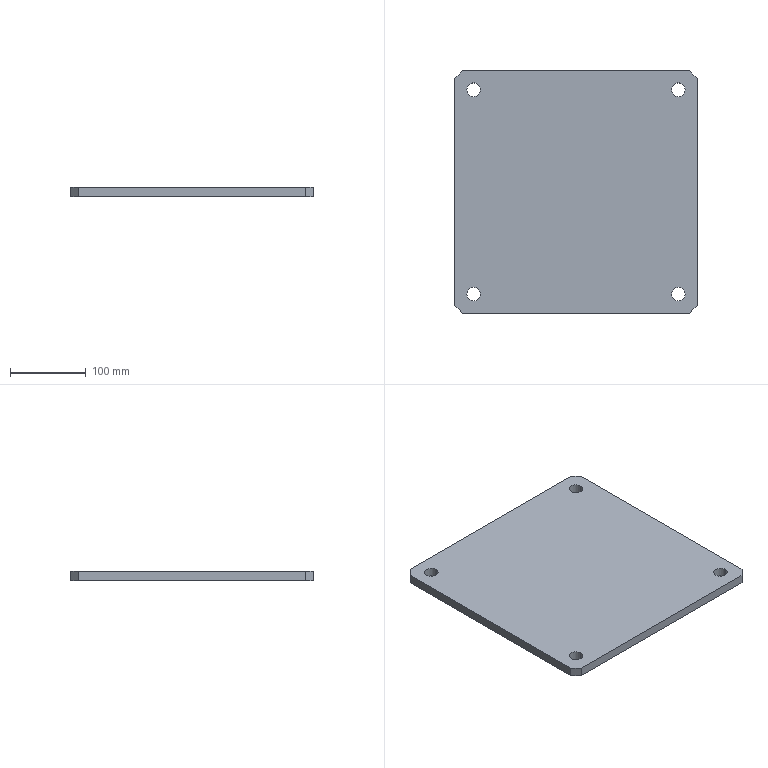Part | STEP file | PN_0109 Mount electronic clip vibrating disc base plate | 1 solid | 18 faces | box 320 x 320 x 12 mm | volume 1214185 mm3 | plane 10 | cylinder 8 | commonest cylinder face diameters 18 x8
STEP:
#1=CARTESIAN_POINT('',(0.,0.,0.));
#2=DIRECTION('',(0.,0.,1.));
#3=DIRECTION('',(1.,0.,0.));
#4=AXIS2_PLACEMENT_3D('',#1,#2,#3);
#5=CARTESIAN_POINT('',(144.,-135.,0.));
#6=VERTEX_POINT('',#5);
#7=CARTESIAN_POINT('',(144.,-135.,12.));
#8=VERTEX_POINT('',#7);
#9=CARTESIAN_POINT('',(144.,-135.,12.));
#10=DIRECTION('',(0.,0.,1.));
#11=VECTOR('',#10,1.);
#12=LINE('',#9,#11);
#13=CARTESIAN_POINT('',(135.,-135.,12.));
#14=DIRECTION('',(0.,0.,1.));
#15=DIRECTION('',(1.,0.,0.));
#16=AXIS2_PLACEMENT_3D('',#13,#14,#15);
#17=CYLINDRICAL_SURFACE('',#16,9.);
#18=CARTESIAN_POINT('',(6.283,0.));
#19=DIRECTION('',(0.,1.));
#20=VECTOR('',#19,1.);
#21=LINE('',#18,#20);
#22=(GEOMETRIC_REPRESENTATION_CONTEXT(2)PARAMETRIC_REPRESENTATION_CONTEXT()REPRESENTATION_CONTEXT('',''));
#23=DEFINITIONAL_REPRESENTATION('',(#21),#22);
#24=PCURVE('',#17,#23);
#25=CARTESIAN_POINT('',(135.,-135.,12.));
#26=DIRECTION('',(0.,0.,1.));
#27=DIRECTION('',(1.,0.,0.));
#28=AXIS2_PLACEMENT_3D('',#25,#26,#27);
#29=CYLINDRICAL_SURFACE('',#28,9.);
#30=CARTESIAN_POINT('',(0.,0.));
#31=DIRECTION('',(0.,1.));
#32=VECTOR('',#31,1.);
#33=LINE('',#30,#32);
#34=(GEOMETRIC_REPRESENTATION_CONTEXT(2)PARAMETRIC_REPRESENTATION_CONTEXT()REPRESENTATION_CONTEXT('',''));
#35=DEFINITIONAL_REPRESENTATION('',(#33),#34);
#36=PCURVE('',#29,#35);
#37=SURFACE_CURVE('',#12,(#24,#36),.PCURVE_S1.);
#38=EDGE_CURVE('',#6,#8,#37,.T.);
#39=ORIENTED_EDGE('',*,*,#38,.T.);
#40=CARTESIAN_POINT('',(126.,-135.,12.));
#41=VERTEX_POINT('',#40);
#42=CARTESIAN_POINT('',(135.,-135.,12.));
#43=DIRECTION('',(0.,0.,1.));
#44=DIRECTION('',(1.,0.,0.));
#45=AXIS2_PLACEMENT_3D('',#42,#43,#44);
#46=CIRCLE('',#45,9.);
#47=CARTESIAN_POINT('',(0.,0.));
#48=DIRECTION('',(1.,0.));
#49=VECTOR('',#48,1.);
#50=LINE('',#47,#49);
#51=(GEOMETRIC_REPRESENTATION_CONTEXT(2)PARAMETRIC_REPRESENTATION_CONTEXT()REPRESENTATION_CONTEXT('',''));
#52=DEFINITIONAL_REPRESENTATION('',(#50),#51);
#53=PCURVE('',#17,#52);
#54=CARTESIAN_POINT('',(0.,0.,12.));
#55=DIRECTION('',(0.,0.,-1.));
#56=DIRECTION('',(-1.,0.,0.));
#57=AXIS2_PLACEMENT_3D('',#54,#55,#56);
#58=PLANE('',#57);
#59=CARTESIAN_POINT('',(-144.,-135.));
#60=CARTESIAN_POINT('',(-144.,-119.412));
#61=CARTESIAN_POINT('',(-130.5,-127.206));
#62=CARTESIAN_POINT('',(-117.,-135.));
#63=CARTESIAN_POINT('',(-130.5,-142.794));
#64=CARTESIAN_POINT('',(-144.,-150.588));
#65=CARTESIAN_POINT('',(-144.,-135.));
#66=(BOUNDED_CURVE()B_SPLINE_CURVE(2,(#59,#60,#61,#62,#63,#64,#65),.UNSPECIFIED.,.T.,.F.)B_SPLINE_CURVE_WITH_KNOTS((1,2,2,2,2,1),(-2.094,0.,2.094,4.189,6.283,8.378),.UNSPECIFIED.)CURVE()GEOMETRIC_REPRESENTATION_ITEM()RATIONAL_B_SPLINE_CURVE((1.,0.5,1.,0.5,1.,0.5,1.))REPRESENTATION_ITEM(''));
#67=(GEOMETRIC_REPRESENTATION_CONTEXT(2)PARAMETRIC_REPRESENTATION_CONTEXT()REPRESENTATION_CONTEXT('',''));
#68=DEFINITIONAL_REPRESENTATION('',(#66),#67);
#69=PCURVE('',#58,#68);
#70=SURFACE_CURVE('',#46,(#53,#69),.PCURVE_S1.);
#71=EDGE_CURVE('',#41,#8,#70,.T.);
#72=ORIENTED_EDGE('',*,*,#71,.F.);
#73=CARTESIAN_POINT('',(126.,-135.,0.));
#74=VERTEX_POINT('',#73);
#75=CARTESIAN_POINT('',(126.,-135.,12.));
#76=DIRECTION('',(0.,0.,1.));
#77=VECTOR('',#76,1.);
#78=LINE('',#75,#77);
#79=CARTESIAN_POINT('',(3.142,0.));
#80=DIRECTION('',(0.,1.));
#81=VECTOR('',#80,1.);
#82=LINE('',#79,#81);
#83=(GEOMETRIC_REPRESENTATION_CONTEXT(2)PARAMETRIC_REPRESENTATION_CONTEXT()REPRESENTATION_CONTEXT('',''));
#84=DEFINITIONAL_REPRESENTATION('',(#82),#83);
#85=PCURVE('',#17,#84);
#86=CARTESIAN_POINT('',(3.142,0.));
#87=DIRECTION('',(0.,1.));
#88=VECTOR('',#87,1.);
#89=LINE('',#86,#88);
#90=(GEOMETRIC_REPRESENTATION_CONTEXT(2)PARAMETRIC_REPRESENTATION_CONTEXT()REPRESENTATION_CONTEXT('',''));
#91=DEFINITIONAL_REPRESENTATION('',(#89),#90);
#92=PCURVE('',#29,#91);
#93=SURFACE_CURVE('',#78,(#85,#92),.PCURVE_S1.);
#94=EDGE_CURVE('',#74,#41,#93,.T.);
#95=ORIENTED_EDGE('',*,*,#94,.F.);
#96=CARTESIAN_POINT('',(135.,-135.,0.));
#97=DIRECTION('',(0.,0.,-1.));
#98=DIRECTION('',(-1.,0.,0.));
#99=AXIS2_PLACEMENT_3D('',#96,#97,#98);
#100=CIRCLE('',#99,9.);
#101=CARTESIAN_POINT('',(9.425,-12.));
#102=DIRECTION('',(-1.,0.));
#103=VECTOR('',#102,1.);
#104=LINE('',#101,#103);
#105=(GEOMETRIC_REPRESENTATION_CONTEXT(2)PARAMETRIC_REPRESENTATION_CONTEXT()REPRESENTATION_CONTEXT('',''));
#106=DEFINITIONAL_REPRESENTATION('',(#104),#105);
#107=PCURVE('',#17,#106);
#108=CARTESIAN_POINT('',(0.,0.,0.));
#109=DIRECTION('',(0.,0.,-1.));
#110=DIRECTION('',(-1.,0.,0.));
#111=AXIS2_PLACEMENT_3D('',#108,#109,#110);
#112=PLANE('',#111);
#113=CARTESIAN_POINT('',(-135.,-135.));
#114=DIRECTION('',(1.,0.));
#115=AXIS2_PLACEMENT_2D('',#113,#114);
#116=CIRCLE('',#115,9.);
#117=(GEOMETRIC_REPRESENTATION_CONTEXT(2)PARAMETRIC_REPRESENTATION_CONTEXT()REPRESENTATION_CONTEXT('',''));
#118=DEFINITIONAL_REPRESENTATION('',(#116),#117);
#119=PCURVE('',#112,#118);
#120=SURFACE_CURVE('',#100,(#107,#119),.PCURVE_S1.);
#121=EDGE_CURVE('',#6,#74,#120,.T.);
#122=ORIENTED_EDGE('',*,*,#121,.F.);
#123=EDGE_LOOP('',(#39,#72,#95,#122));
#124=FACE_BOUND('',#123,.F.);
#125=ADVANCED_FACE('',(#124),#17,.F.);
#126=CARTESIAN_POINT('',(144.,135.,0.));
#127=VERTEX_POINT('',#126);
#128=CARTESIAN_POINT('',(144.,135.,12.));
#129=VERTEX_POINT('',#128);
#130=CARTESIAN_POINT('',(144.,135.,12.));
#131=DIRECTION('',(0.,0.,1.));
#132=VECTOR('',#131,1.);
#133=LINE('',#130,#132);
#134=CARTESIAN_POINT('',(135.,135.,12.));
#135=DIRECTION('',(0.,0.,1.));
#136=DIRECTION('',(1.,0.,0.));
#137=AXIS2_PLACEMENT_3D('',#134,#135,#136);
#138=CYLINDRICAL_SURFACE('',#137,9.);
#139=CARTESIAN_POINT('',(6.283,0.));
#140=DIRECTION('',(0.,1.));
#141=VECTOR('',#140,1.);
#142=LINE('',#139,#141);
#143=(GEOMETRIC_REPRESENTATION_CONTEXT(2)PARAMETRIC_REPRESENTATION_CONTEXT()REPRESENTATION_CONTEXT('',''));
#144=DEFINITIONAL_REPRESENTATION('',(#142),#143);
#145=PCURVE('',#138,#144);
#146=CARTESIAN_POINT('',(135.,135.,12.));
#147=DIRECTION('',(0.,0.,1.));
#148=DIRECTION('',(1.,0.,0.));
#149=AXIS2_PLACEMENT_3D('',#146,#147,#148);
#150=CYLINDRICAL_SURFACE('',#149,9.);
#151=CARTESIAN_POINT('',(0.,0.));
#152=DIRECTION('',(0.,1.));
#153=VECTOR('',#152,1.);
#154=LINE('',#151,#153);
#155=(GEOMETRIC_REPRESENTATION_CONTEXT(2)PARAMETRIC_REPRESENTATION_CONTEXT()REPRESENTATION_CONTEXT('',''));
#156=DEFINITIONAL_REPRESENTATION('',(#154),#155);
#157=PCURVE('',#150,#156);
#158=SURFACE_CURVE('',#133,(#145,#157),.PCURVE_S1.);
#159=EDGE_CURVE('',#127,#129,#158,.T.);
#160=ORIENTED_EDGE('',*,*,#159,.T.);
#161=CARTESIAN_POINT('',(126.,135.,12.));
#162=VERTEX_POINT('',#161);
#163=CARTESIAN_POINT('',(135.,135.,12.));
#164=DIRECTION('',(0.,0.,1.));
#165=DIRECTION('',(1.,0.,0.));
#166=AXIS2_PLACEMENT_3D('',#163,#164,#165);
#167=CIRCLE('',#166,9.);
#168=CARTESIAN_POINT('',(0.,0.));
#169=DIRECTION('',(1.,0.));
#170=VECTOR('',#169,1.);
#171=LINE('',#168,#170);
#172=(GEOMETRIC_REPRESENTATION_CONTEXT(2)PARAMETRIC_REPRESENTATION_CONTEXT()REPRESENTATION_CONTEXT('',''));
#173=DEFINITIONAL_REPRESENTATION('',(#171),#172);
#174=PCURVE('',#138,#173);
#175=CARTESIAN_POINT('',(-144.,135.));
#176=CARTESIAN_POINT('',(-144.,150.588));
#177=CARTESIAN_POINT('',(-130.5,142.794));
#178=CARTESIAN_POINT('',(-117.,135.));
#179=CARTESIAN_POINT('',(-130.5,127.206));
#180=CARTESIAN_POINT('',(-144.,119.412));
#181=CARTESIAN_POINT('',(-144.,135.));
#182=(BOUNDED_CURVE()B_SPLINE_CURVE(2,(#175,#176,#177,#178,#179,#180,#181),.UNSPECIFIED.,.T.,.F.)B_SPLINE_CURVE_WITH_KNOTS((1,2,2,2,2,1),(-2.094,0.,2.094,4.189,6.283,8.378),.UNSPECIFIED.)CURVE()GEOMETRIC_REPRESENTATION_ITEM()RATIONAL_B_SPLINE_CURVE((1.,0.5,1.,0.5,1.,0.5,1.))REPRESENTATION_ITEM(''));
#183=(GEOMETRIC_REPRESENTATION_CONTEXT(2)PARAMETRIC_REPRESENTATION_CONTEXT()REPRESENTATION_CONTEXT('',''));
#184=DEFINITIONAL_REPRESENTATION('',(#182),#183);
#185=PCURVE('',#58,#184);
#186=SURFACE_CURVE('',#167,(#174,#185),.PCURVE_S1.);
#187=EDGE_CURVE('',#162,#129,#186,.T.);
#188=ORIENTED_EDGE('',*,*,#187,.F.);
#189=CARTESIAN_POINT('',(126.,135.,0.));
#190=VERTEX_POINT('',#189);
#191=CARTESIAN_POINT('',(126.,135.,12.));
#192=DIRECTION('',(0.,0.,1.));
#193=VECTOR('',#192,1.);
#194=LINE('',#191,#193);
#195=CARTESIAN_POINT('',(3.142,0.));
#196=DIRECTION('',(0.,1.));
#197=VECTOR('',#196,1.);
#198=LINE('',#195,#197);
#199=(GEOMETRIC_REPRESENTATION_CONTEXT(2)PARAMETRIC_REPRESENTATION_CONTEXT()REPRESENTATION_CONTEXT('',''));
#200=DEFINITIONAL_REPRESENTATION('',(#198),#199);
#201=PCURVE('',#138,#200);
#202=CARTESIAN_POINT('',(3.142,0.));
#203=DIRECTION('',(0.,1.));
#204=VECTOR('',#203,1.);
#205=LINE('',#202,#204);
#206=(GEOMETRIC_REPRESENTATION_CONTEXT(2)PARAMETRIC_REPRESENTATION_CONTEXT()REPRESENTATION_CONTEXT('',''));
#207=DEFINITIONAL_REPRESENTATION('',(#205),#206);
#208=PCURVE('',#150,#207);
#209=SURFACE_CURVE('',#194,(#201,#208),.PCURVE_S1.);
#210=EDGE_CURVE('',#190,#162,#209,.T.);
#211=ORIENTED_EDGE('',*,*,#210,.F.);
#212=CARTESIAN_POINT('',(135.,135.,0.));
#213=DIRECTION('',(0.,0.,-1.));
#214=DIRECTION('',(-1.,0.,0.));
#215=AXIS2_PLACEMENT_3D('',#212,#213,#214);
#216=CIRCLE('',#215,9.);
#217=CARTESIAN_POINT('',(9.425,-12.));
#218=DIRECTION('',(-1.,0.));
#219=VECTOR('',#218,1.);
#220=LINE('',#217,#219);
#221=(GEOMETRIC_REPRESENTATION_CONTEXT(2)PARAMETRIC_REPRESENTATION_CONTEXT()REPRESENTATION_CONTEXT('',''));
#222=DEFINITIONAL_REPRESENTATION('',(#220),#221);
#223=PCURVE('',#138,#222);
#224=CARTESIAN_POINT('',(-135.,135.));
#225=DIRECTION('',(1.,0.));
#226=AXIS2_PLACEMENT_2D('',#224,#225);
#227=CIRCLE('',#226,9.);
#228=(GEOMETRIC_REPRESENTATION_CONTEXT(2)PARAMETRIC_REPRESENTATION_CONTEXT()REPRESENTATION_CONTEXT('',''));
#229=DEFINITIONAL_REPRESENTATION('',(#227),#228);
#230=PCURVE('',#112,#229);
#231=SURFACE_CURVE('',#216,(#223,#230),.PCURVE_S1.);
#232=EDGE_CURVE('',#127,#190,#231,.T.);
#233=ORIENTED_EDGE('',*,*,#232,.F.);
#234=EDGE_LOOP('',(#160,#188,#211,#233));
#235=FACE_BOUND('',#234,.F.);
#236=ADVANCED_FACE('',(#235),#138,.F.);
#237=CARTESIAN_POINT('',(-126.,-135.,0.));
#238=VERTEX_POINT('',#237);
#239=CARTESIAN_POINT('',(-126.,-135.,12.));
#240=VERTEX_POINT('',#239);
#241=CARTESIAN_POINT('',(-126.,-135.,12.));
#242=DIRECTION('',(0.,0.,1.));
#243=VECTOR('',#242,1.);
#244=LINE('',#241,#243);
#245=CARTESIAN_POINT('',(-135.,-135.,12.));
#246=DIRECTION('',(0.,0.,1.));
#247=DIRECTION('',(1.,0.,0.));
#248=AXIS2_PLACEMENT_3D('',#245,#246,#247);
#249=CYLINDRICAL_SURFACE('',#248,9.);
#250=CARTESIAN_POINT('',(6.283,0.));
#251=DIRECTION('',(0.,1.));
#252=VECTOR('',#251,1.);
#253=LINE('',#250,#252);
#254=(GEOMETRIC_REPRESENTATION_CONTEXT(2)PARAMETRIC_REPRESENTATION_CONTEXT()REPRESENTATION_CONTEXT('',''));
#255=DEFINITIONAL_REPRESENTATION('',(#253),#254);
#256=PCURVE('',#249,#255);
#257=CARTESIAN_POINT('',(-135.,-135.,12.));
#258=DIRECTION('',(0.,0.,1.));
#259=DIRECTION('',(1.,0.,0.));
#260=AXIS2_PLACEMENT_3D('',#257,#258,#259);
#261=CYLINDRICAL_SURFACE('',#260,9.);
#262=CARTESIAN_POINT('',(0.,0.));
#263=DIRECTION('',(0.,1.));
#264=VECTOR('',#263,1.);
#265=LINE('',#262,#264);
#266=(GEOMETRIC_REPRESENTATION_CONTEXT(2)PARAMETRIC_REPRESENTATION_CONTEXT()REPRESENTATION_CONTEXT('',''));
#267=DEFINITIONAL_REPRESENTATION('',(#265),#266);
#268=PCURVE('',#261,#267);
#269=SURFACE_CURVE('',#244,(#256,#268),.PCURVE_S1.);
#270=EDGE_CURVE('',#238,#240,#269,.T.);
#271=ORIENTED_EDGE('',*,*,#270,.T.);
#272=CARTESIAN_POINT('',(-144.,-135.,12.));
#273=VERTEX_POINT('',#272);
#274=CARTESIAN_POINT('',(-135.,-135.,12.));
#275=DIRECTION('',(0.,0.,1.));
#276=DIRECTION('',(1.,0.,0.));
#277=AXIS2_PLACEMENT_3D('',#274,#275,#276);
#278=CIRCLE('',#277,9.);
#279=CARTESIAN_POINT('',(0.,0.));
#280=DIRECTION('',(1.,0.));
#281=VECTOR('',#280,1.);
#282=LINE('',#279,#281);
#283=(GEOMETRIC_REPRESENTATION_CONTEXT(2)PARAMETRIC_REPRESENTATION_CONTEXT()REPRESENTATION_CONTEXT('',''));
#284=DEFINITIONAL_REPRESENTATION('',(#282),#283);
#285=PCURVE('',#249,#284);
#286=CARTESIAN_POINT('',(126.,-135.));
#287=CARTESIAN_POINT('',(126.,-119.412));
#288=CARTESIAN_POINT('',(139.5,-127.206));
#289=CARTESIAN_POINT('',(153.,-135.));
#290=CARTESIAN_POINT('',(139.5,-142.794));
#291=CARTESIAN_POINT('',(126.,-150.588));
#292=CARTESIAN_POINT('',(126.,-135.));
#293=(BOUNDED_CURVE()B_SPLINE_CURVE(2,(#286,#287,#288,#289,#290,#291,#292),.UNSPECIFIED.,.T.,.F.)B_SPLINE_CURVE_WITH_KNOTS((1,2,2,2,2,1),(-2.094,0.,2.094,4.189,6.283,8.378),.UNSPECIFIED.)CURVE()GEOMETRIC_REPRESENTATION_ITEM()RATIONAL_B_SPLINE_CURVE((1.,0.5,1.,0.5,1.,0.5,1.))REPRESENTATION_ITEM(''));
#294=(GEOMETRIC_REPRESENTATION_CONTEXT(2)PARAMETRIC_REPRESENTATION_CONTEXT()REPRESENTATION_CONTEXT('',''));
#295=DEFINITIONAL_REPRESENTATION('',(#293),#294);
#296=PCURVE('',#58,#295);
#297=SURFACE_CURVE('',#278,(#285,#296),.PCURVE_S1.);
#298=EDGE_CURVE('',#273,#240,#297,.T.);
#299=ORIENTED_EDGE('',*,*,#298,.F.);
#300=CARTESIAN_POINT('',(-144.,-135.,0.));
#301=VERTEX_POINT('',#300);
#302=CARTESIAN_POINT('',(-144.,-135.,12.));
#303=DIRECTION('',(0.,0.,1.));
#304=VECTOR('',#303,1.);
#305=LINE('',#302,#304);
#306=CARTESIAN_POINT('',(3.142,0.));
#307=DIRECTION('',(0.,1.));
#308=VECTOR('',#307,1.);
#309=LINE('',#306,#308);
#310=(GEOMETRIC_REPRESENTATION_CONTEXT(2)PARAMETRIC_REPRESENTATION_CONTEXT()REPRESENTATION_CONTEXT('',''));
#311=DEFINITIONAL_REPRESENTATION('',(#309),#310);
#312=PCURVE('',#249,#311);
#313=CARTESIAN_POINT('',(3.142,0.));
#314=DIRECTION('',(0.,1.));
#315=VECTOR('',#314,1.);
#316=LINE('',#313,#315);
#317=(GEOMETRIC_REPRESENTATION_CONTEXT(2)PARAMETRIC_REPRESENTATION_CONTEXT()REPRESENTATION_CONTEXT('',''));
#318=DEFINITIONAL_REPRESENTATION('',(#316),#317);
#319=PCURVE('',#261,#318);
#320=SURFACE_CURVE('',#305,(#312,#319),.PCURVE_S1.);
#321=EDGE_CURVE('',#301,#273,#320,.T.);
#322=ORIENTED_EDGE('',*,*,#321,.F.);
#323=CARTESIAN_POINT('',(-135.,-135.,0.));
#324=DIRECTION('',(0.,0.,-1.));
#325=DIRECTION('',(-1.,0.,0.));
#326=AXIS2_PLACEMENT_3D('',#323,#324,#325);
#327=CIRCLE('',#326,9.);
#328=CARTESIAN_POINT('',(9.425,-12.));
#329=DIRECTION('',(-1.,0.));
#330=VECTOR('',#329,1.);
#331=LINE('',#328,#330);
#332=(GEOMETRIC_REPRESENTATION_CONTEXT(2)PARAMETRIC_REPRESENTATION_CONTEXT()REPRESENTATION_CONTEXT('',''));
#333=DEFINITIONAL_REPRESENTATION('',(#331),#332);
#334=PCURVE('',#249,#333);
#335=CARTESIAN_POINT('',(135.,-135.));
#336=DIRECTION('',(1.,0.));
#337=AXIS2_PLACEMENT_2D('',#335,#336);
#338=CIRCLE('',#337,9.);
#339=(GEOMETRIC_REPRESENTATION_CONTEXT(2)PARAMETRIC_REPRESENTATION_CONTEXT()REPRESENTATION_CONTEXT('',''));
#340=DEFINITIONAL_REPRESENTATION('',(#338),#339);
#341=PCURVE('',#112,#340);
#342=SURFACE_CURVE('',#327,(#334,#341),.PCURVE_S1.);
#343=EDGE_CURVE('',#238,#301,#342,.T.);
#344=ORIENTED_EDGE('',*,*,#343,.F.);
#345=EDGE_LOOP('',(#271,#299,#322,#344));
#346=FACE_BOUND('',#345,.F.);
#347=ADVANCED_FACE('',(#346),#249,.F.);
#348=CARTESIAN_POINT('',(-126.,135.,0.));
#349=VERTEX_POINT('',#348);
#350=CARTESIAN_POINT('',(-126.,135.,12.));
#351=VERTEX_POINT('',#350);
#352=CARTESIAN_POINT('',(-126.,135.,12.));
#353=DIRECTION('',(0.,0.,1.));
#354=VECTOR('',#353,1.);
#355=LINE('',#352,#354);
#356=CARTESIAN_POINT('',(-135.,135.,12.));
#357=DIRECTION('',(0.,0.,1.));
#358=DIRECTION('',(1.,0.,0.));
#359=AXIS2_PLACEMENT_3D('',#356,#357,#358);
#360=CYLINDRICAL_SURFACE('',#359,9.);
#361=CARTESIAN_POINT('',(6.283,0.));
#362=DIRECTION('',(0.,1.));
#363=VECTOR('',#362,1.);
#364=LINE('',#361,#363);
#365=(GEOMETRIC_REPRESENTATION_CONTEXT(2)PARAMETRIC_REPRESENTATION_CONTEXT()REPRESENTATION_CONTEXT('',''));
#366=DEFINITIONAL_REPRESENTATION('',(#364),#365);
#367=PCURVE('',#360,#366);
#368=CARTESIAN_POINT('',(-135.,135.,12.));
#369=DIRECTION('',(0.,0.,1.));
#370=DIRECTION('',(1.,0.,0.));
#371=AXIS2_PLACEMENT_3D('',#368,#369,#370);
#372=CYLINDRICAL_SURFACE('',#371,9.);
#373=CARTESIAN_POINT('',(0.,0.));
#374=DIRECTION('',(0.,1.));
#375=VECTOR('',#374,1.);
#376=LINE('',#373,#375);
#377=(GEOMETRIC_REPRESENTATION_CONTEXT(2)PARAMETRIC_REPRESENTATION_CONTEXT()REPRESENTATION_CONTEXT('',''));
#378=DEFINITIONAL_REPRESENTATION('',(#376),#377);
#379=PCURVE('',#372,#378);
#380=SURFACE_CURVE('',#355,(#367,#379),.PCURVE_S1.);
#381=EDGE_CURVE('',#349,#351,#380,.T.);
#382=ORIENTED_EDGE('',*,*,#381,.T.);
#383=CARTESIAN_POINT('',(-144.,135.,12.));
#384=VERTEX_POINT('',#383);
#385=CARTESIAN_POINT('',(-135.,135.,12.));
#386=DIRECTION('',(0.,0.,1.));
#387=DIRECTION('',(1.,0.,0.));
#388=AXIS2_PLACEMENT_3D('',#385,#386,#387);
#389=CIRCLE('',#388,9.);
#390=CARTESIAN_POINT('',(0.,0.));
#391=DIRECTION('',(1.,0.));
#392=VECTOR('',#391,1.);
#393=LINE('',#390,#392);
#394=(GEOMETRIC_REPRESENTATION_CONTEXT(2)PARAMETRIC_REPRESENTATION_CONTEXT()REPRESENTATION_CONTEXT('',''));
#395=DEFINITIONAL_REPRESENTATION('',(#393),#394);
#396=PCURVE('',#360,#395);
#397=CARTESIAN_POINT('',(126.,135.));
#398=CARTESIAN_POINT('',(126.,150.588));
#399=CARTESIAN_POINT('',(139.5,142.794));
#400=CARTESIAN_POINT('',(153.,135.));
#401=CARTESIAN_POINT('',(139.5,127.206));
#402=CARTESIAN_POINT('',(126.,119.412));
#403=CARTESIAN_POINT('',(126.,135.));
#404=(BOUNDED_CURVE()B_SPLINE_CURVE(2,(#397,#398,#399,#400,#401,#402,#403),.UNSPECIFIED.,.T.,.F.)B_SPLINE_CURVE_WITH_KNOTS((1,2,2,2,2,1),(-2.094,0.,2.094,4.189,6.283,8.378),.UNSPECIFIED.)CURVE()GEOMETRIC_REPRESENTATION_ITEM()RATIONAL_B_SPLINE_CURVE((1.,0.5,1.,0.5,1.,0.5,1.))REPRESENTATION_ITEM(''));
#405=(GEOMETRIC_REPRESENTATION_CONTEXT(2)PARAMETRIC_REPRESENTATION_CONTEXT()REPRESENTATION_CONTEXT('',''));
#406=DEFINITIONAL_REPRESENTATION('',(#404),#405);
#407=PCURVE('',#58,#406);
#408=SURFACE_CURVE('',#389,(#396,#407),.PCURVE_S1.);
#409=EDGE_CURVE('',#384,#351,#408,.T.);
#410=ORIENTED_EDGE('',*,*,#409,.F.);
#411=CARTESIAN_POINT('',(-144.,135.,0.));
#412=VERTEX_POINT('',#411);
#413=CARTESIAN_POINT('',(-144.,135.,12.));
#414=DIRECTION('',(0.,0.,1.));
#415=VECTOR('',#414,1.);
#416=LINE('',#413,#415);
#417=CARTESIAN_POINT('',(3.142,0.));
#418=DIRECTION('',(0.,1.));
#419=VECTOR('',#418,1.);
#420=LINE('',#417,#419);
#421=(GEOMETRIC_REPRESENTATION_CONTEXT(2)PARAMETRIC_REPRESENTATION_CONTEXT()REPRESENTATION_CONTEXT('',''));
#422=DEFINITIONAL_REPRESENTATION('',(#420),#421);
#423=PCURVE('',#360,#422);
#424=CARTESIAN_POINT('',(3.142,0.));
#425=DIRECTION('',(0.,1.));
#426=VECTOR('',#425,1.);
#427=LINE('',#424,#426);
#428=(GEOMETRIC_REPRESENTATION_CONTEXT(2)PARAMETRIC_REPRESENTATION_CONTEXT()REPRESENTATION_CONTEXT('',''));
#429=DEFINITIONAL_REPRESENTATION('',(#427),#428);
#430=PCURVE('',#372,#429);
#431=SURFACE_CURVE('',#416,(#423,#430),.PCURVE_S1.);
#432=EDGE_CURVE('',#412,#384,#431,.T.);
#433=ORIENTED_EDGE('',*,*,#432,.F.);
#434=CARTESIAN_POINT('',(-135.,135.,0.));
#435=DIRECTION('',(0.,0.,-1.));
#436=DIRECTION('',(-1.,0.,0.));
#437=AXIS2_PLACEMENT_3D('',#434,#435,#436);
#438=CIRCLE('',#437,9.);
#439=CARTESIAN_POINT('',(9.425,-12.));
#440=DIRECTION('',(-1.,0.));
#441=VECTOR('',#440,1.);
#442=LINE('',#439,#441);
#443=(GEOMETRIC_REPRESENTATION_CONTEXT(2)PARAMETRIC_REPRESENTATION_CONTEXT()REPRESENTATION_CONTEXT('',''));
#444=DEFINITIONAL_REPRESENTATION('',(#442),#443);
#445=PCURVE('',#360,#444);
#446=CARTESIAN_POINT('',(135.,135.));
#447=DIRECTION('',(1.,0.));
#448=AXIS2_PLACEMENT_2D('',#446,#447);
#449=CIRCLE('',#448,9.);
#450=(GEOMETRIC_REPRESENTATION_CONTEXT(2)PARAMETRIC_REPRESENTATION_CONTEXT()REPRESENTATION_CONTEXT('',''));
#451=DEFINITIONAL_REPRESENTATION('',(#449),#450);
#452=PCURVE('',#112,#451);
#453=SURFACE_CURVE('',#438,(#445,#452),.PCURVE_S1.);
#454=EDGE_CURVE('',#349,#412,#453,.T.);
#455=ORIENTED_EDGE('',*,*,#454,.F.);
#456=EDGE_LOOP('',(#382,#410,#433,#455));
#457=FACE_BOUND('',#456,.F.);
#458=ADVANCED_FACE('',(#457),#360,.F.);
#459=CARTESIAN_POINT('',(160.,-150.,0.));
#460=VERTEX_POINT('',#459);
#461=CARTESIAN_POINT('',(160.,150.,0.));
#462=VERTEX_POINT('',#461);
#463=CARTESIAN_POINT('',(160.,-160.,0.));
#464=DIRECTION('',(0.,1.,0.));
#465=VECTOR('',#464,1.);
#466=LINE('',#463,#465);
#467=CARTESIAN_POINT('',(160.,-160.,12.));
#468=DIRECTION('',(-1.,0.,0.));
#469=DIRECTION('',(0.,0.,1.));
#470=AXIS2_PLACEMENT_3D('',#467,#468,#469);
#471=PLANE('',#470);
#472=CARTESIAN_POINT('',(-12.,0.));
#473=DIRECTION('',(0.,1.));
#474=VECTOR('',#473,1.);
#475=LINE('',#472,#474);
#476=(GEOMETRIC_REPRESENTATION_CONTEXT(2)PARAMETRIC_REPRESENTATION_CONTEXT()REPRESENTATION_CONTEXT('',''));
#477=DEFINITIONAL_REPRESENTATION('',(#475),#476);
#478=PCURVE('',#471,#477);
#479=CARTESIAN_POINT('',(-160.,-160.));
#480=DIRECTION('',(0.,1.));
#481=VECTOR('',#480,1.);
#482=LINE('',#479,#481);
#483=(GEOMETRIC_REPRESENTATION_CONTEXT(2)PARAMETRIC_REPRESENTATION_CONTEXT()REPRESENTATION_CONTEXT('',''));
#484=DEFINITIONAL_REPRESENTATION('',(#482),#483);
#485=PCURVE('',#112,#484);
#486=SURFACE_CURVE('',#466,(#478,#485),.PCURVE_S1.);
#487=EDGE_CURVE('',#460,#462,#486,.T.);
#488=ORIENTED_EDGE('',*,*,#487,.T.);
#489=CARTESIAN_POINT('',(160.,150.,12.));
#490=VERTEX_POINT('',#489);
#491=CARTESIAN_POINT('',(160.,150.,12.));
#492=DIRECTION('',(0.,0.,1.));
#493=VECTOR('',#492,1.);
#494=LINE('',#491,#493);
#495=CARTESIAN_POINT('',(0.,310.));
#496=DIRECTION('',(1.,0.));
#497=VECTOR('',#496,1.);
#498=LINE('',#495,#497);
#499=(GEOMETRIC_REPRESENTATION_CONTEXT(2)PARAMETRIC_REPRESENTATION_CONTEXT()REPRESENTATION_CONTEXT('',''));
#500=DEFINITIONAL_REPRESENTATION('',(#498),#499);
#501=PCURVE('',#471,#500);
#502=CARTESIAN_POINT('',(150.,160.,12.));
#503=DIRECTION('',(-0.7071,-0.7071,0.));
#504=DIRECTION('',(0.,0.,-1.));
#505=AXIS2_PLACEMENT_3D('',#502,#503,#504);
#506=PLANE('',#505);
#507=CARTESIAN_POINT('',(0.,14.142));
#508=DIRECTION('',(-1.,0.));
#509=VECTOR('',#508,1.);
#510=LINE('',#507,#509);
#511=(GEOMETRIC_REPRESENTATION_CONTEXT(2)PARAMETRIC_REPRESENTATION_CONTEXT()REPRESENTATION_CONTEXT('',''));
#512=DEFINITIONAL_REPRESENTATION('',(#510),#511);
#513=PCURVE('',#506,#512);
#514=SURFACE_CURVE('',#494,(#501,#513),.PCURVE_S1.);
#515=EDGE_CURVE('',#462,#490,#514,.T.);
#516=ORIENTED_EDGE('',*,*,#515,.T.);
#517=CARTESIAN_POINT('',(160.,-150.,12.));
#518=VERTEX_POINT('',#517);
#519=CARTESIAN_POINT('',(160.,-160.,12.));
#520=DIRECTION('',(0.,1.,0.));
#521=VECTOR('',#520,1.);
#522=LINE('',#519,#521);
#523=CARTESIAN_POINT('',(0.,0.));
#524=DIRECTION('',(0.,1.));
#525=VECTOR('',#524,1.);
#526=LINE('',#523,#525);
#527=(GEOMETRIC_REPRESENTATION_CONTEXT(2)PARAMETRIC_REPRESENTATION_CONTEXT()REPRESENTATION_CONTEXT('',''));
#528=DEFINITIONAL_REPRESENTATION('',(#526),#527);
#529=PCURVE('',#471,#528);
#530=CARTESIAN_POINT('',(-160.,-160.));
#531=DIRECTION('',(0.,1.));
#532=VECTOR('',#531,1.);
#533=LINE('',#530,#532);
#534=(GEOMETRIC_REPRESENTATION_CONTEXT(2)PARAMETRIC_REPRESENTATION_CONTEXT()REPRESENTATION_CONTEXT('',''));
#535=DEFINITIONAL_REPRESENTATION('',(#533),#534);
#536=PCURVE('',#58,#535);
#537=SURFACE_CURVE('',#522,(#529,#536),.PCURVE_S1.);
#538=EDGE_CURVE('',#518,#490,#537,.T.);
#539=ORIENTED_EDGE('',*,*,#538,.F.);
#540=CARTESIAN_POINT('',(160.,-150.,12.));
#541=DIRECTION('',(0.,0.,-1.));
#542=VECTOR('',#541,1.);
#543=LINE('',#540,#542);
#544=CARTESIAN_POINT('',(0.,10.));
#545=DIRECTION('',(-1.,0.));
#546=VECTOR('',#545,1.);
#547=LINE('',#544,#546);
#548=(GEOMETRIC_REPRESENTATION_CONTEXT(2)PARAMETRIC_REPRESENTATION_CONTEXT()REPRESENTATION_CONTEXT('',''));
#549=DEFINITIONAL_REPRESENTATION('',(#547),#548);
#550=PCURVE('',#471,#549);
#551=CARTESIAN_POINT('',(160.,-150.,12.));
#552=DIRECTION('',(-0.7071,0.7071,0.));
#553=DIRECTION('',(0.,0.,-1.));
#554=AXIS2_PLACEMENT_3D('',#551,#552,#553);
#555=PLANE('',#554);
#556=CARTESIAN_POINT('',(0.,0.));
#557=DIRECTION('',(1.,0.));
#558=VECTOR('',#557,1.);
#559=LINE('',#556,#558);
#560=(GEOMETRIC_REPRESENTATION_CONTEXT(2)PARAMETRIC_REPRESENTATION_CONTEXT()REPRESENTATION_CONTEXT('',''));
#561=DEFINITIONAL_REPRESENTATION('',(#559),#560);
#562=PCURVE('',#555,#561);
#563=SURFACE_CURVE('',#543,(#550,#562),.PCURVE_S1.);
#564=EDGE_CURVE('',#518,#460,#563,.T.);
#565=ORIENTED_EDGE('',*,*,#564,.T.);
#566=EDGE_LOOP('',(#488,#516,#539,#565));
#567=FACE_BOUND('',#566,.T.);
#568=ADVANCED_FACE('',(#567),#471,.F.);
#569=CARTESIAN_POINT('',(150.,160.,0.));
#570=VERTEX_POINT('',#569);
#571=CARTESIAN_POINT('',(-150.,160.,0.));
#572=VERTEX_POINT('',#571);
#573=CARTESIAN_POINT('',(-160.,160.,0.));
#574=DIRECTION('',(-1.,0.,0.));
#575=VECTOR('',#574,1.);
#576=LINE('',#573,#575);
#577=CARTESIAN_POINT('',(-160.,160.,12.));
#578=DIRECTION('',(0.,-1.,0.));
#579=DIRECTION('',(0.,0.,-1.));
#580=AXIS2_PLACEMENT_3D('',#577,#578,#579);
#581=PLANE('',#580);
#582=CARTESIAN_POINT('',(12.,0.));
#583=DIRECTION('',(0.,-1.));
#584=VECTOR('',#583,1.);
#585=LINE('',#582,#584);
#586=(GEOMETRIC_REPRESENTATION_CONTEXT(2)PARAMETRIC_REPRESENTATION_CONTEXT()REPRESENTATION_CONTEXT('',''));
#587=DEFINITIONAL_REPRESENTATION('',(#585),#586);
#588=PCURVE('',#581,#587);
#589=CARTESIAN_POINT('',(160.,160.));
#590=DIRECTION('',(1.,0.));
#591=VECTOR('',#590,1.);
#592=LINE('',#589,#591);
#593=(GEOMETRIC_REPRESENTATION_CONTEXT(2)PARAMETRIC_REPRESENTATION_CONTEXT()REPRESENTATION_CONTEXT('',''));
#594=DEFINITIONAL_REPRESENTATION('',(#592),#593);
#595=PCURVE('',#112,#594);
#596=SURFACE_CURVE('',#576,(#588,#595),.PCURVE_S1.);
#597=EDGE_CURVE('',#570,#572,#596,.T.);
#598=ORIENTED_EDGE('',*,*,#597,.T.);
#599=CARTESIAN_POINT('',(-150.,160.,12.));
#600=VERTEX_POINT('',#599);
#601=CARTESIAN_POINT('',(-150.,160.,12.));
#602=DIRECTION('',(0.,0.,1.));
#603=VECTOR('',#602,1.);
#604=LINE('',#601,#603);
#605=CARTESIAN_POINT('',(0.,10.));
#606=DIRECTION('',(-1.,0.));
#607=VECTOR('',#606,1.);
#608=LINE('',#605,#607);
#609=(GEOMETRIC_REPRESENTATION_CONTEXT(2)PARAMETRIC_REPRESENTATION_CONTEXT()REPRESENTATION_CONTEXT('',''));
#610=DEFINITIONAL_REPRESENTATION('',(#608),#609);
#611=PCURVE('',#581,#610);
#612=CARTESIAN_POINT('',(-160.,150.,12.));
#613=DIRECTION('',(0.7071,-0.7071,0.));
#614=DIRECTION('',(0.,0.,-1.));
#615=AXIS2_PLACEMENT_3D('',#612,#613,#614);
#616=PLANE('',#615);
#617=CARTESIAN_POINT('',(0.,14.142));
#618=DIRECTION('',(-1.,0.));
#619=VECTOR('',#618,1.);
#620=LINE('',#617,#619);
#621=(GEOMETRIC_REPRESENTATION_CONTEXT(2)PARAMETRIC_REPRESENTATION_CONTEXT()REPRESENTATION_CONTEXT('',''));
#622=DEFINITIONAL_REPRESENTATION('',(#620),#621);
#623=PCURVE('',#616,#622);
#624=SURFACE_CURVE('',#604,(#611,#623),.PCURVE_S1.);
#625=EDGE_CURVE('',#572,#600,#624,.T.);
#626=ORIENTED_EDGE('',*,*,#625,.T.);
#627=CARTESIAN_POINT('',(150.,160.,12.));
#628=VERTEX_POINT('',#627);
#629=CARTESIAN_POINT('',(-160.,160.,12.));
#630=DIRECTION('',(-1.,0.,0.));
#631=VECTOR('',#630,1.);
#632=LINE('',#629,#631);
#633=CARTESIAN_POINT('',(0.,0.));
#634=DIRECTION('',(0.,-1.));
#635=VECTOR('',#634,1.);
#636=LINE('',#633,#635);
#637=(GEOMETRIC_REPRESENTATION_CONTEXT(2)PARAMETRIC_REPRESENTATION_CONTEXT()REPRESENTATION_CONTEXT('',''));
#638=DEFINITIONAL_REPRESENTATION('',(#636),#637);
#639=PCURVE('',#581,#638);
#640=CARTESIAN_POINT('',(160.,160.));
#641=DIRECTION('',(1.,0.));
#642=VECTOR('',#641,1.);
#643=LINE('',#640,#642);
#644=(GEOMETRIC_REPRESENTATION_CONTEXT(2)PARAMETRIC_REPRESENTATION_CONTEXT()REPRESENTATION_CONTEXT('',''));
#645=DEFINITIONAL_REPRESENTATION('',(#643),#644);
#646=PCURVE('',#58,#645);
#647=SURFACE_CURVE('',#632,(#639,#646),.PCURVE_S1.);
#648=EDGE_CURVE('',#628,#600,#647,.T.);
#649=ORIENTED_EDGE('',*,*,#648,.F.);
#650=CARTESIAN_POINT('',(150.,160.,12.));
#651=DIRECTION('',(0.,0.,-1.));
#652=VECTOR('',#651,1.);
#653=LINE('',#650,#652);
#654=CARTESIAN_POINT('',(0.,310.));
#655=DIRECTION('',(1.,0.));
#656=VECTOR('',#655,1.);
#657=LINE('',#654,#656);
#658=(GEOMETRIC_REPRESENTATION_CONTEXT(2)PARAMETRIC_REPRESENTATION_CONTEXT()REPRESENTATION_CONTEXT('',''));
#659=DEFINITIONAL_REPRESENTATION('',(#657),#658);
#660=PCURVE('',#581,#659);
#661=CARTESIAN_POINT('',(0.,0.));
#662=DIRECTION('',(1.,0.));
#663=VECTOR('',#662,1.);
#664=LINE('',#661,#663);
#665=(GEOMETRIC_REPRESENTATION_CONTEXT(2)PARAMETRIC_REPRESENTATION_CONTEXT()REPRESENTATION_CONTEXT('',''));
#666=DEFINITIONAL_REPRESENTATION('',(#664),#665);
#667=PCURVE('',#506,#666);
#668=SURFACE_CURVE('',#653,(#660,#667),.PCURVE_S1.);
#669=EDGE_CURVE('',#628,#570,#668,.T.);
#670=ORIENTED_EDGE('',*,*,#669,.T.);
#671=EDGE_LOOP('',(#598,#626,#649,#670));
#672=FACE_BOUND('',#671,.T.);
#673=ADVANCED_FACE('',(#672),#581,.F.);
#674=CARTESIAN_POINT('',(-160.,150.,12.));
#675=VERTEX_POINT('',#674);
#676=CARTESIAN_POINT('',(-160.,-150.,12.));
#677=VERTEX_POINT('',#676);
#678=CARTESIAN_POINT('',(-160.,-160.,12.));
#679=DIRECTION('',(0.,-1.,0.));
#680=VECTOR('',#679,1.);
#681=LINE('',#678,#680);
#682=CARTESIAN_POINT('',(-160.,-160.,12.));
#683=DIRECTION('',(1.,0.,0.));
#684=DIRECTION('',(0.,0.,-1.));
#685=AXIS2_PLACEMENT_3D('',#682,#683,#684);
#686=PLANE('',#685);
#687=CARTESIAN_POINT('',(0.,0.));
#688=DIRECTION('',(0.,-1.));
#689=VECTOR('',#688,1.);
#690=LINE('',#687,#689);
#691=(GEOMETRIC_REPRESENTATION_CONTEXT(2)PARAMETRIC_REPRESENTATION_CONTEXT()REPRESENTATION_CONTEXT('',''));
#692=DEFINITIONAL_REPRESENTATION('',(#690),#691);
#693=PCURVE('',#686,#692);
#694=CARTESIAN_POINT('',(160.,-160.));
#695=DIRECTION('',(0.,-1.));
#696=VECTOR('',#695,1.);
#697=LINE('',#694,#696);
#698=(GEOMETRIC_REPRESENTATION_CONTEXT(2)PARAMETRIC_REPRESENTATION_CONTEXT()REPRESENTATION_CONTEXT('',''));
#699=DEFINITIONAL_REPRESENTATION('',(#697),#698);
#700=PCURVE('',#58,#699);
#701=SURFACE_CURVE('',#681,(#693,#700),.PCURVE_S1.);
#702=EDGE_CURVE('',#675,#677,#701,.T.);
#703=ORIENTED_EDGE('',*,*,#702,.F.);
#704=CARTESIAN_POINT('',(-160.,150.,0.));
#705=VERTEX_POINT('',#704);
#706=CARTESIAN_POINT('',(-160.,150.,12.));
#707=DIRECTION('',(0.,0.,-1.));
#708=VECTOR('',#707,1.);
#709=LINE('',#706,#708);
#710=CARTESIAN_POINT('',(0.,310.));
#711=DIRECTION('',(1.,0.));
#712=VECTOR('',#711,1.);
#713=LINE('',#710,#712);
#714=(GEOMETRIC_REPRESENTATION_CONTEXT(2)PARAMETRIC_REPRESENTATION_CONTEXT()REPRESENTATION_CONTEXT('',''));
#715=DEFINITIONAL_REPRESENTATION('',(#713),#714);
#716=PCURVE('',#686,#715);
#717=CARTESIAN_POINT('',(0.,0.));
#718=DIRECTION('',(1.,0.));
#719=VECTOR('',#718,1.);
#720=LINE('',#717,#719);
#721=(GEOMETRIC_REPRESENTATION_CONTEXT(2)PARAMETRIC_REPRESENTATION_CONTEXT()REPRESENTATION_CONTEXT('',''));
#722=DEFINITIONAL_REPRESENTATION('',(#720),#721);
#723=PCURVE('',#616,#722);
#724=SURFACE_CURVE('',#709,(#716,#723),.PCURVE_S1.);
#725=EDGE_CURVE('',#675,#705,#724,.T.);
#726=ORIENTED_EDGE('',*,*,#725,.T.);
#727=CARTESIAN_POINT('',(-160.,-150.,0.));
#728=VERTEX_POINT('',#727);
#729=CARTESIAN_POINT('',(-160.,-160.,0.));
#730=DIRECTION('',(0.,-1.,0.));
#731=VECTOR('',#730,1.);
#732=LINE('',#729,#731);
#733=CARTESIAN_POINT('',(12.,0.));
#734=DIRECTION('',(0.,-1.));
#735=VECTOR('',#734,1.);
#736=LINE('',#733,#735);
#737=(GEOMETRIC_REPRESENTATION_CONTEXT(2)PARAMETRIC_REPRESENTATION_CONTEXT()REPRESENTATION_CONTEXT('',''));
#738=DEFINITIONAL_REPRESENTATION('',(#736),#737);
#739=PCURVE('',#686,#738);
#740=CARTESIAN_POINT('',(160.,-160.));
#741=DIRECTION('',(0.,-1.));
#742=VECTOR('',#741,1.);
#743=LINE('',#740,#742);
#744=(GEOMETRIC_REPRESENTATION_CONTEXT(2)PARAMETRIC_REPRESENTATION_CONTEXT()REPRESENTATION_CONTEXT('',''));
#745=DEFINITIONAL_REPRESENTATION('',(#743),#744);
#746=PCURVE('',#112,#745);
#747=SURFACE_CURVE('',#732,(#739,#746),.PCURVE_S1.);
#748=EDGE_CURVE('',#705,#728,#747,.T.);
#749=ORIENTED_EDGE('',*,*,#748,.T.);
#750=CARTESIAN_POINT('',(-160.,-150.,12.));
#751=DIRECTION('',(0.,0.,1.));
#752=VECTOR('',#751,1.);
#753=LINE('',#750,#752);
#754=CARTESIAN_POINT('',(0.,10.));
#755=DIRECTION('',(-1.,0.));
#756=VECTOR('',#755,1.);
#757=LINE('',#754,#756);
#758=(GEOMETRIC_REPRESENTATION_CONTEXT(2)PARAMETRIC_REPRESENTATION_CONTEXT()REPRESENTATION_CONTEXT('',''));
#759=DEFINITIONAL_REPRESENTATION('',(#757),#758);
#760=PCURVE('',#686,#759);
#761=CARTESIAN_POINT('',(-150.,-160.,12.));
#762=DIRECTION('',(0.7071,0.7071,0.));
#763=DIRECTION('',(0.,0.,-1.));
#764=AXIS2_PLACEMENT_3D('',#761,#762,#763);
#765=PLANE('',#764);
#766=CARTESIAN_POINT('',(0.,14.142));
#767=DIRECTION('',(-1.,0.));
#768=VECTOR('',#767,1.);
#769=LINE('',#766,#768);
#770=(GEOMETRIC_REPRESENTATION_CONTEXT(2)PARAMETRIC_REPRESENTATION_CONTEXT()REPRESENTATION_CONTEXT('',''));
#771=DEFINITIONAL_REPRESENTATION('',(#769),#770);
#772=PCURVE('',#765,#771);
#773=SURFACE_CURVE('',#753,(#760,#772),.PCURVE_S1.);
#774=EDGE_CURVE('',#728,#677,#773,.T.);
#775=ORIENTED_EDGE('',*,*,#774,.T.);
#776=EDGE_LOOP('',(#703,#726,#749,#775));
#777=FACE_BOUND('',#776,.T.);
#778=ADVANCED_FACE('',(#777),#686,.F.);
#779=CARTESIAN_POINT('',(-150.,-160.,0.));
#780=VERTEX_POINT('',#779);
#781=CARTESIAN_POINT('',(150.,-160.,0.));
#782=VERTEX_POINT('',#781);
#783=CARTESIAN_POINT('',(-160.,-160.,0.));
#784=DIRECTION('',(1.,0.,0.));
#785=VECTOR('',#784,1.);
#786=LINE('',#783,#785);
#787=CARTESIAN_POINT('',(-160.,-160.,12.));
#788=DIRECTION('',(0.,1.,0.));
#789=DIRECTION('',(0.,0.,1.));
#790=AXIS2_PLACEMENT_3D('',#787,#788,#789);
#791=PLANE('',#790);
#792=CARTESIAN_POINT('',(-12.,0.));
#793=DIRECTION('',(0.,1.));
#794=VECTOR('',#793,1.);
#795=LINE('',#792,#794);
#796=(GEOMETRIC_REPRESENTATION_CONTEXT(2)PARAMETRIC_REPRESENTATION_CONTEXT()REPRESENTATION_CONTEXT('',''));
#797=DEFINITIONAL_REPRESENTATION('',(#795),#796);
#798=PCURVE('',#791,#797);
#799=CARTESIAN_POINT('',(160.,-160.));
#800=DIRECTION('',(-1.,0.));
#801=VECTOR('',#800,1.);
#802=LINE('',#799,#801);
#803=(GEOMETRIC_REPRESENTATION_CONTEXT(2)PARAMETRIC_REPRESENTATION_CONTEXT()REPRESENTATION_CONTEXT('',''));
#804=DEFINITIONAL_REPRESENTATION('',(#802),#803);
#805=PCURVE('',#112,#804);
#806=SURFACE_CURVE('',#786,(#798,#805),.PCURVE_S1.);
#807=EDGE_CURVE('',#780,#782,#806,.T.);
#808=ORIENTED_EDGE('',*,*,#807,.T.);
#809=CARTESIAN_POINT('',(150.,-160.,12.));
#810=VERTEX_POINT('',#809);
#811=CARTESIAN_POINT('',(150.,-160.,12.));
#812=DIRECTION('',(0.,0.,1.));
#813=VECTOR('',#812,1.);
#814=LINE('',#811,#813);
#815=CARTESIAN_POINT('',(0.,310.));
#816=DIRECTION('',(1.,0.));
#817=VECTOR('',#816,1.);
#818=LINE('',#815,#817);
#819=(GEOMETRIC_REPRESENTATION_CONTEXT(2)PARAMETRIC_REPRESENTATION_CONTEXT()REPRESENTATION_CONTEXT('',''));
#820=DEFINITIONAL_REPRESENTATION('',(#818),#819);
#821=PCURVE('',#791,#820);
#822=CARTESIAN_POINT('',(0.,14.142));
#823=DIRECTION('',(-1.,0.));
#824=VECTOR('',#823,1.);
#825=LINE('',#822,#824);
#826=(GEOMETRIC_REPRESENTATION_CONTEXT(2)PARAMETRIC_REPRESENTATION_CONTEXT()REPRESENTATION_CONTEXT('',''));
#827=DEFINITIONAL_REPRESENTATION('',(#825),#826);
#828=PCURVE('',#555,#827);
#829=SURFACE_CURVE('',#814,(#821,#828),.PCURVE_S1.);
#830=EDGE_CURVE('',#782,#810,#829,.T.);
#831=ORIENTED_EDGE('',*,*,#830,.T.);
#832=CARTESIAN_POINT('',(-150.,-160.,12.));
#833=VERTEX_POINT('',#832);
#834=CARTESIAN_POINT('',(-160.,-160.,12.));
#835=DIRECTION('',(1.,0.,0.));
#836=VECTOR('',#835,1.);
#837=LINE('',#834,#836);
#838=CARTESIAN_POINT('',(0.,0.));
#839=DIRECTION('',(0.,1.));
#840=VECTOR('',#839,1.);
#841=LINE('',#838,#840);
#842=(GEOMETRIC_REPRESENTATION_CONTEXT(2)PARAMETRIC_REPRESENTATION_CONTEXT()REPRESENTATION_CONTEXT('',''));
#843=DEFINITIONAL_REPRESENTATION('',(#841),#842);
#844=PCURVE('',#791,#843);
#845=CARTESIAN_POINT('',(160.,-160.));
#846=DIRECTION('',(-1.,0.));
#847=VECTOR('',#846,1.);
#848=LINE('',#845,#847);
#849=(GEOMETRIC_REPRESENTATION_CONTEXT(2)PARAMETRIC_REPRESENTATION_CONTEXT()REPRESENTATION_CONTEXT('',''));
#850=DEFINITIONAL_REPRESENTATION('',(#848),#849);
#851=PCURVE('',#58,#850);
#852=SURFACE_CURVE('',#837,(#844,#851),.PCURVE_S1.);
#853=EDGE_CURVE('',#833,#810,#852,.T.);
#854=ORIENTED_EDGE('',*,*,#853,.F.);
#855=CARTESIAN_POINT('',(-150.,-160.,12.));
#856=DIRECTION('',(0.,0.,-1.));
#857=VECTOR('',#856,1.);
#858=LINE('',#855,#857);
#859=CARTESIAN_POINT('',(0.,10.));
#860=DIRECTION('',(-1.,0.));
#861=VECTOR('',#860,1.);
#862=LINE('',#859,#861);
#863=(GEOMETRIC_REPRESENTATION_CONTEXT(2)PARAMETRIC_REPRESENTATION_CONTEXT()REPRESENTATION_CONTEXT('',''));
#864=DEFINITIONAL_REPRESENTATION('',(#862),#863);
#865=PCURVE('',#791,#864);
#866=CARTESIAN_POINT('',(0.,0.));
#867=DIRECTION('',(1.,0.));
#868=VECTOR('',#867,1.);
#869=LINE('',#866,#868);
#870=(GEOMETRIC_REPRESENTATION_CONTEXT(2)PARAMETRIC_REPRESENTATION_CONTEXT()REPRESENTATION_CONTEXT('',''));
#871=DEFINITIONAL_REPRESENTATION('',(#869),#870);
#872=PCURVE('',#765,#871);
#873=SURFACE_CURVE('',#858,(#865,#872),.PCURVE_S1.);
#874=EDGE_CURVE('',#833,#780,#873,.T.);
#875=ORIENTED_EDGE('',*,*,#874,.T.);
#876=EDGE_LOOP('',(#808,#831,#854,#875));
#877=FACE_BOUND('',#876,.T.);
#878=ADVANCED_FACE('',(#877),#791,.F.);
#879=CARTESIAN_POINT('',(-135.,-135.,12.));
#880=DIRECTION('',(0.,0.,1.));
#881=DIRECTION('',(1.,0.,0.));
#882=AXIS2_PLACEMENT_3D('',#879,#880,#881);
#883=CIRCLE('',#882,9.);
#884=CARTESIAN_POINT('',(126.,-135.));
#885=CARTESIAN_POINT('',(126.,-119.412));
#886=CARTESIAN_POINT('',(139.5,-127.206));
#887=CARTESIAN_POINT('',(153.,-135.));
#888=CARTESIAN_POINT('',(139.5,-142.794));
#889=CARTESIAN_POINT('',(126.,-150.588));
#890=CARTESIAN_POINT('',(126.,-135.));
#891=(BOUNDED_CURVE()B_SPLINE_CURVE(2,(#884,#885,#886,#887,#888,#889,#890),.UNSPECIFIED.,.T.,.F.)B_SPLINE_CURVE_WITH_KNOTS((1,2,2,2,2,1),(-2.094,0.,2.094,4.189,6.283,8.378),.UNSPECIFIED.)CURVE()GEOMETRIC_REPRESENTATION_ITEM()RATIONAL_B_SPLINE_CURVE((1.,0.5,1.,0.5,1.,0.5,1.))REPRESENTATION_ITEM(''));
#892=(GEOMETRIC_REPRESENTATION_CONTEXT(2)PARAMETRIC_REPRESENTATION_CONTEXT()REPRESENTATION_CONTEXT('',''));
#893=DEFINITIONAL_REPRESENTATION('',(#891),#892);
#894=PCURVE('',#58,#893);
#895=CARTESIAN_POINT('',(0.,0.));
#896=DIRECTION('',(1.,0.));
#897=VECTOR('',#896,1.);
#898=LINE('',#895,#897);
#899=(GEOMETRIC_REPRESENTATION_CONTEXT(2)PARAMETRIC_REPRESENTATION_CONTEXT()REPRESENTATION_CONTEXT('',''));
#900=DEFINITIONAL_REPRESENTATION('',(#898),#899);
#901=PCURVE('',#261,#900);
#902=SURFACE_CURVE('',#883,(#894,#901),.PCURVE_S1.);
#903=EDGE_CURVE('',#240,#273,#902,.T.);
#904=ORIENTED_EDGE('',*,*,#903,.F.);
#905=ORIENTED_EDGE('',*,*,#298,.F.);
#906=EDGE_LOOP('',(#904,#905));
#907=FACE_BOUND('',#906,.T.);
#908=CARTESIAN_POINT('',(-135.,135.,12.));
#909=DIRECTION('',(0.,0.,1.));
#910=DIRECTION('',(1.,0.,0.));
#911=AXIS2_PLACEMENT_3D('',#908,#909,#910);
#912=CIRCLE('',#911,9.);
#913=CARTESIAN_POINT('',(126.,135.));
#914=CARTESIAN_POINT('',(126.,150.588));
#915=CARTESIAN_POINT('',(139.5,142.794));
#916=CARTESIAN_POINT('',(153.,135.));
#917=CARTESIAN_POINT('',(139.5,127.206));
#918=CARTESIAN_POINT('',(126.,119.412));
#919=CARTESIAN_POINT('',(126.,135.));
#920=(BOUNDED_CURVE()B_SPLINE_CURVE(2,(#913,#914,#915,#916,#917,#918,#919),.UNSPECIFIED.,.T.,.F.)B_SPLINE_CURVE_WITH_KNOTS((1,2,2,2,2,1),(-2.094,0.,2.094,4.189,6.283,8.378),.UNSPECIFIED.)CURVE()GEOMETRIC_REPRESENTATION_ITEM()RATIONAL_B_SPLINE_CURVE((1.,0.5,1.,0.5,1.,0.5,1.))REPRESENTATION_ITEM(''));
#921=(GEOMETRIC_REPRESENTATION_CONTEXT(2)PARAMETRIC_REPRESENTATION_CONTEXT()REPRESENTATION_CONTEXT('',''));
#922=DEFINITIONAL_REPRESENTATION('',(#920),#921);
#923=PCURVE('',#58,#922);
#924=CARTESIAN_POINT('',(0.,0.));
#925=DIRECTION('',(1.,0.));
#926=VECTOR('',#925,1.);
#927=LINE('',#924,#926);
#928=(GEOMETRIC_REPRESENTATION_CONTEXT(2)PARAMETRIC_REPRESENTATION_CONTEXT()REPRESENTATION_CONTEXT('',''));
#929=DEFINITIONAL_REPRESENTATION('',(#927),#928);
#930=PCURVE('',#372,#929);
#931=SURFACE_CURVE('',#912,(#923,#930),.PCURVE_S1.);
#932=EDGE_CURVE('',#351,#384,#931,.T.);
#933=ORIENTED_EDGE('',*,*,#932,.F.);
#934=ORIENTED_EDGE('',*,*,#409,.F.);
#935=EDGE_LOOP('',(#933,#934));
#936=FACE_BOUND('',#935,.T.);
#937=ORIENTED_EDGE('',*,*,#648,.T.);
#938=CARTESIAN_POINT('',(-160.,150.,12.));
#939=DIRECTION('',(-0.7071,-0.7071,0.));
#940=VECTOR('',#939,1.);
#941=LINE('',#938,#940);
#942=CARTESIAN_POINT('',(160.,150.));
#943=DIRECTION('',(0.7071,-0.7071));
#944=VECTOR('',#943,1.);
#945=LINE('',#942,#944);
#946=(GEOMETRIC_REPRESENTATION_CONTEXT(2)PARAMETRIC_REPRESENTATION_CONTEXT()REPRESENTATION_CONTEXT('',''));
#947=DEFINITIONAL_REPRESENTATION('',(#945),#946);
#948=PCURVE('',#58,#947);
#949=CARTESIAN_POINT('',(0.,0.));
#950=DIRECTION('',(0.,-1.));
#951=VECTOR('',#950,1.);
#952=LINE('',#949,#951);
#953=(GEOMETRIC_REPRESENTATION_CONTEXT(2)PARAMETRIC_REPRESENTATION_CONTEXT()REPRESENTATION_CONTEXT('',''));
#954=DEFINITIONAL_REPRESENTATION('',(#952),#953);
#955=PCURVE('',#616,#954);
#956=SURFACE_CURVE('',#941,(#948,#955),.PCURVE_S1.);
#957=EDGE_CURVE('',#600,#675,#956,.T.);
#958=ORIENTED_EDGE('',*,*,#957,.T.);
#959=ORIENTED_EDGE('',*,*,#702,.T.);
#960=CARTESIAN_POINT('',(-150.,-160.,12.));
#961=DIRECTION('',(0.7071,-0.7071,0.));
#962=VECTOR('',#961,1.);
#963=LINE('',#960,#962);
#964=CARTESIAN_POINT('',(150.,-160.));
#965=DIRECTION('',(-0.7071,-0.7071));
#966=VECTOR('',#965,1.);
#967=LINE('',#964,#966);
#968=(GEOMETRIC_REPRESENTATION_CONTEXT(2)PARAMETRIC_REPRESENTATION_CONTEXT()REPRESENTATION_CONTEXT('',''));
#969=DEFINITIONAL_REPRESENTATION('',(#967),#968);
#970=PCURVE('',#58,#969);
#971=CARTESIAN_POINT('',(0.,0.));
#972=DIRECTION('',(0.,-1.));
#973=VECTOR('',#972,1.);
#974=LINE('',#971,#973);
#975=(GEOMETRIC_REPRESENTATION_CONTEXT(2)PARAMETRIC_REPRESENTATION_CONTEXT()REPRESENTATION_CONTEXT('',''));
#976=DEFINITIONAL_REPRESENTATION('',(#974),#975);
#977=PCURVE('',#765,#976);
#978=SURFACE_CURVE('',#963,(#970,#977),.PCURVE_S1.);
#979=EDGE_CURVE('',#677,#833,#978,.T.);
#980=ORIENTED_EDGE('',*,*,#979,.T.);
#981=ORIENTED_EDGE('',*,*,#853,.T.);
#982=CARTESIAN_POINT('',(160.,-150.,12.));
#983=DIRECTION('',(0.7071,0.7071,0.));
#984=VECTOR('',#983,1.);
#985=LINE('',#982,#984);
#986=CARTESIAN_POINT('',(-160.,-150.));
#987=DIRECTION('',(-0.7071,0.7071));
#988=VECTOR('',#987,1.);
#989=LINE('',#986,#988);
#990=(GEOMETRIC_REPRESENTATION_CONTEXT(2)PARAMETRIC_REPRESENTATION_CONTEXT()REPRESENTATION_CONTEXT('',''));
#991=DEFINITIONAL_REPRESENTATION('',(#989),#990);
#992=PCURVE('',#58,#991);
#993=CARTESIAN_POINT('',(0.,0.));
#994=DIRECTION('',(0.,-1.));
#995=VECTOR('',#994,1.);
#996=LINE('',#993,#995);
#997=(GEOMETRIC_REPRESENTATION_CONTEXT(2)PARAMETRIC_REPRESENTATION_CONTEXT()REPRESENTATION_CONTEXT('',''));
#998=DEFINITIONAL_REPRESENTATION('',(#996),#997);
#999=PCURVE('',#555,#998);
#1000=SURFACE_CURVE('',#985,(#992,#999),.PCURVE_S1.);
#1001=EDGE_CURVE('',#810,#518,#1000,.T.);
#1002=ORIENTED_EDGE('',*,*,#1001,.T.);
#1003=ORIENTED_EDGE('',*,*,#538,.T.);
#1004=CARTESIAN_POINT('',(150.,160.,12.));
#1005=DIRECTION('',(-0.7071,0.7071,0.));
#1006=VECTOR('',#1005,1.);
#1007=LINE('',#1004,#1006);
#1008=CARTESIAN_POINT('',(-150.,160.));
#1009=DIRECTION('',(0.7071,0.7071));
#1010=VECTOR('',#1009,1.);
#1011=LINE('',#1008,#1010);
#1012=(GEOMETRIC_REPRESENTATION_CONTEXT(2)PARAMETRIC_REPRESENTATION_CONTEXT()REPRESENTATION_CONTEXT('',''));
#1013=DEFINITIONAL_REPRESENTATION('',(#1011),#1012);
#1014=PCURVE('',#58,#1013);
#1015=CARTESIAN_POINT('',(0.,0.));
#1016=DIRECTION('',(0.,-1.));
#1017=VECTOR('',#1016,1.);
#1018=LINE('',#1015,#1017);
#1019=(GEOMETRIC_REPRESENTATION_CONTEXT(2)PARAMETRIC_REPRESENTATION_CONTEXT()REPRESENTATION_CONTEXT('',''));
#1020=DEFINITIONAL_REPRESENTATION('',(#1018),#1019);
#1021=PCURVE('',#506,#1020);
#1022=SURFACE_CURVE('',#1007,(#1014,#1021),.PCURVE_S1.);
#1023=EDGE_CURVE('',#490,#628,#1022,.T.);
#1024=ORIENTED_EDGE('',*,*,#1023,.T.);
#1025=EDGE_LOOP('',(#937,#958,#959,#980,#981,#1002,#1003,#1024));
#1026=FACE_BOUND('',#1025,.T.);
#1027=CARTESIAN_POINT('',(135.,135.,12.));
#1028=DIRECTION('',(0.,0.,1.));
#1029=DIRECTION('',(1.,0.,0.));
#1030=AXIS2_PLACEMENT_3D('',#1027,#1028,#1029);
#1031=CIRCLE('',#1030,9.);
#1032=CARTESIAN_POINT('',(-144.,135.));
#1033=CARTESIAN_POINT('',(-144.,150.588));
#1034=CARTESIAN_POINT('',(-130.5,142.794));
#1035=CARTESIAN_POINT('',(-117.,135.));
#1036=CARTESIAN_POINT('',(-130.5,127.206));
#1037=CARTESIAN_POINT('',(-144.,119.412));
#1038=CARTESIAN_POINT('',(-144.,135.));
#1039=(BOUNDED_CURVE()B_SPLINE_CURVE(2,(#1032,#1033,#1034,#1035,#1036,#1037,#1038),.UNSPECIFIED.,.T.,.F.)B_SPLINE_CURVE_WITH_KNOTS((1,2,2,2,2,1),(-2.094,0.,2.094,4.189,6.283,8.378),.UNSPECIFIED.)CURVE()GEOMETRIC_REPRESENTATION_ITEM()RATIONAL_B_SPLINE_CURVE((1.,0.5,1.,0.5,1.,0.5,1.))REPRESENTATION_ITEM(''));
#1040=(GEOMETRIC_REPRESENTATION_CONTEXT(2)PARAMETRIC_REPRESENTATION_CONTEXT()REPRESENTATION_CONTEXT('',''));
#1041=DEFINITIONAL_REPRESENTATION('',(#1039),#1040);
#1042=PCURVE('',#58,#1041);
#1043=CARTESIAN_POINT('',(0.,0.));
#1044=DIRECTION('',(1.,0.));
#1045=VECTOR('',#1044,1.);
#1046=LINE('',#1043,#1045);
#1047=(GEOMETRIC_REPRESENTATION_CONTEXT(2)PARAMETRIC_REPRESENTATION_CONTEXT()REPRESENTATION_CONTEXT('',''));
#1048=DEFINITIONAL_REPRESENTATION('',(#1046),#1047);
#1049=PCURVE('',#150,#1048);
#1050=SURFACE_CURVE('',#1031,(#1042,#1049),.PCURVE_S1.);
#1051=EDGE_CURVE('',#129,#162,#1050,.T.);
#1052=ORIENTED_EDGE('',*,*,#1051,.F.);
#1053=ORIENTED_EDGE('',*,*,#187,.F.);
#1054=EDGE_LOOP('',(#1052,#1053));
#1055=FACE_BOUND('',#1054,.T.);
#1056=CARTESIAN_POINT('',(135.,-135.,12.));
#1057=DIRECTION('',(0.,0.,1.));
#1058=DIRECTION('',(1.,0.,0.));
#1059=AXIS2_PLACEMENT_3D('',#1056,#1057,#1058);
#1060=CIRCLE('',#1059,9.);
#1061=CARTESIAN_POINT('',(-144.,-135.));
#1062=CARTESIAN_POINT('',(-144.,-119.412));
#1063=CARTESIAN_POINT('',(-130.5,-127.206));
#1064=CARTESIAN_POINT('',(-117.,-135.));
#1065=CARTESIAN_POINT('',(-130.5,-142.794));
#1066=CARTESIAN_POINT('',(-144.,-150.588));
#1067=CARTESIAN_POINT('',(-144.,-135.));
#1068=(BOUNDED_CURVE()B_SPLINE_CURVE(2,(#1061,#1062,#1063,#1064,#1065,#1066,#1067),.UNSPECIFIED.,.T.,.F.)B_SPLINE_CURVE_WITH_KNOTS((1,2,2,2,2,1),(-2.094,0.,2.094,4.189,6.283,8.378),.UNSPECIFIED.)CURVE()GEOMETRIC_REPRESENTATION_ITEM()RATIONAL_B_SPLINE_CURVE((1.,0.5,1.,0.5,1.,0.5,1.))REPRESENTATION_ITEM(''));
#1069=(GEOMETRIC_REPRESENTATION_CONTEXT(2)PARAMETRIC_REPRESENTATION_CONTEXT()REPRESENTATION_CONTEXT('',''));
#1070=DEFINITIONAL_REPRESENTATION('',(#1068),#1069);
#1071=PCURVE('',#58,#1070);
#1072=CARTESIAN_POINT('',(0.,0.));
#1073=DIRECTION('',(1.,0.));
#1074=VECTOR('',#1073,1.);
#1075=LINE('',#1072,#1074);
#1076=(GEOMETRIC_REPRESENTATION_CONTEXT(2)PARAMETRIC_REPRESENTATION_CONTEXT()REPRESENTATION_CONTEXT('',''));
#1077=DEFINITIONAL_REPRESENTATION('',(#1075),#1076);
#1078=PCURVE('',#29,#1077);
#1079=SURFACE_CURVE('',#1060,(#1071,#1078),.PCURVE_S1.);
#1080=EDGE_CURVE('',#8,#41,#1079,.T.);
#1081=ORIENTED_EDGE('',*,*,#1080,.F.);
#1082=ORIENTED_EDGE('',*,*,#71,.F.);
#1083=EDGE_LOOP('',(#1081,#1082));
#1084=FACE_BOUND('',#1083,.T.);
#1085=ADVANCED_FACE('',(#907,#936,#1026,#1055,#1084),#58,.F.);
#1086=ORIENTED_EDGE('',*,*,#343,.F.);
#1087=CARTESIAN_POINT('',(-135.,-135.,0.));
#1088=DIRECTION('',(0.,0.,-1.));
#1089=DIRECTION('',(-1.,0.,0.));
#1090=AXIS2_PLACEMENT_3D('',#1087,#1088,#1089);
#1091=CIRCLE('',#1090,9.);
#1092=CARTESIAN_POINT('',(135.,-135.));
#1093=DIRECTION('',(1.,0.));
#1094=AXIS2_PLACEMENT_2D('',#1092,#1093);
#1095=CIRCLE('',#1094,9.);
#1096=(GEOMETRIC_REPRESENTATION_CONTEXT(2)PARAMETRIC_REPRESENTATION_CONTEXT()REPRESENTATION_CONTEXT('',''));
#1097=DEFINITIONAL_REPRESENTATION('',(#1095),#1096);
#1098=PCURVE('',#112,#1097);
#1099=CARTESIAN_POINT('',(3.142,-12.));
#1100=DIRECTION('',(-1.,0.));
#1101=VECTOR('',#1100,1.);
#1102=LINE('',#1099,#1101);
#1103=(GEOMETRIC_REPRESENTATION_CONTEXT(2)PARAMETRIC_REPRESENTATION_CONTEXT()REPRESENTATION_CONTEXT('',''));
#1104=DEFINITIONAL_REPRESENTATION('',(#1102),#1103);
#1105=PCURVE('',#261,#1104);
#1106=SURFACE_CURVE('',#1091,(#1098,#1105),.PCURVE_S1.);
#1107=EDGE_CURVE('',#301,#238,#1106,.T.);
#1108=ORIENTED_EDGE('',*,*,#1107,.F.);
#1109=EDGE_LOOP('',(#1086,#1108));
#1110=FACE_BOUND('',#1109,.T.);
#1111=ORIENTED_EDGE('',*,*,#454,.F.);
#1112=CARTESIAN_POINT('',(-135.,135.,0.));
#1113=DIRECTION('',(0.,0.,-1.));
#1114=DIRECTION('',(-1.,0.,0.));
#1115=AXIS2_PLACEMENT_3D('',#1112,#1113,#1114);
#1116=CIRCLE('',#1115,9.);
#1117=CARTESIAN_POINT('',(135.,135.));
#1118=DIRECTION('',(1.,0.));
#1119=AXIS2_PLACEMENT_2D('',#1117,#1118);
#1120=CIRCLE('',#1119,9.);
#1121=(GEOMETRIC_REPRESENTATION_CONTEXT(2)PARAMETRIC_REPRESENTATION_CONTEXT()REPRESENTATION_CONTEXT('',''));
#1122=DEFINITIONAL_REPRESENTATION('',(#1120),#1121);
#1123=PCURVE('',#112,#1122);
#1124=CARTESIAN_POINT('',(3.142,-12.));
#1125=DIRECTION('',(-1.,0.));
#1126=VECTOR('',#1125,1.);
#1127=LINE('',#1124,#1126);
#1128=(GEOMETRIC_REPRESENTATION_CONTEXT(2)PARAMETRIC_REPRESENTATION_CONTEXT()REPRESENTATION_CONTEXT('',''));
#1129=DEFINITIONAL_REPRESENTATION('',(#1127),#1128);
#1130=PCURVE('',#372,#1129);
#1131=SURFACE_CURVE('',#1116,(#1123,#1130),.PCURVE_S1.);
#1132=EDGE_CURVE('',#412,#349,#1131,.T.);
#1133=ORIENTED_EDGE('',*,*,#1132,.F.);
#1134=EDGE_LOOP('',(#1111,#1133));
#1135=FACE_BOUND('',#1134,.T.);
#1136=ORIENTED_EDGE('',*,*,#748,.F.);
#1137=CARTESIAN_POINT('',(-155.,155.,0.));
#1138=DIRECTION('',(0.7071,0.7071,0.));
#1139=VECTOR('',#1138,1.);
#1140=LINE('',#1137,#1139);
#1141=CARTESIAN_POINT('',(155.,155.));
#1142=DIRECTION('',(-0.7071,0.7071));
#1143=VECTOR('',#1142,1.);
#1144=LINE('',#1141,#1143);
#1145=(GEOMETRIC_REPRESENTATION_CONTEXT(2)PARAMETRIC_REPRESENTATION_CONTEXT()REPRESENTATION_CONTEXT('',''));
#1146=DEFINITIONAL_REPRESENTATION('',(#1144),#1145);
#1147=PCURVE('',#112,#1146);
#1148=CARTESIAN_POINT('',(12.,7.071));
#1149=DIRECTION('',(0.,1.));
#1150=VECTOR('',#1149,1.);
#1151=LINE('',#1148,#1150);
#1152=(GEOMETRIC_REPRESENTATION_CONTEXT(2)PARAMETRIC_REPRESENTATION_CONTEXT()REPRESENTATION_CONTEXT('',''));
#1153=DEFINITIONAL_REPRESENTATION('',(#1151),#1152);
#1154=PCURVE('',#616,#1153);
#1155=SURFACE_CURVE('',#1140,(#1147,#1154),.PCURVE_S1.);
#1156=EDGE_CURVE('',#705,#572,#1155,.T.);
#1157=ORIENTED_EDGE('',*,*,#1156,.T.);
#1158=ORIENTED_EDGE('',*,*,#597,.F.);
#1159=CARTESIAN_POINT('',(155.,155.,0.));
#1160=DIRECTION('',(0.7071,-0.7071,0.));
#1161=VECTOR('',#1160,1.);
#1162=LINE('',#1159,#1161);
#1163=CARTESIAN_POINT('',(-155.,155.));
#1164=DIRECTION('',(-0.7071,-0.7071));
#1165=VECTOR('',#1164,1.);
#1166=LINE('',#1163,#1165);
#1167=(GEOMETRIC_REPRESENTATION_CONTEXT(2)PARAMETRIC_REPRESENTATION_CONTEXT()REPRESENTATION_CONTEXT('',''));
#1168=DEFINITIONAL_REPRESENTATION('',(#1166),#1167);
#1169=PCURVE('',#112,#1168);
#1170=CARTESIAN_POINT('',(12.,7.071));
#1171=DIRECTION('',(0.,1.));
#1172=VECTOR('',#1171,1.);
#1173=LINE('',#1170,#1172);
#1174=(GEOMETRIC_REPRESENTATION_CONTEXT(2)PARAMETRIC_REPRESENTATION_CONTEXT()REPRESENTATION_CONTEXT('',''));
#1175=DEFINITIONAL_REPRESENTATION('',(#1173),#1174);
#1176=PCURVE('',#506,#1175);
#1177=SURFACE_CURVE('',#1162,(#1169,#1176),.PCURVE_S1.);
#1178=EDGE_CURVE('',#570,#462,#1177,.T.);
#1179=ORIENTED_EDGE('',*,*,#1178,.T.);
#1180=ORIENTED_EDGE('',*,*,#487,.F.);
#1181=CARTESIAN_POINT('',(155.,-155.,0.));
#1182=DIRECTION('',(-0.7071,-0.7071,0.));
#1183=VECTOR('',#1182,1.);
#1184=LINE('',#1181,#1183);
#1185=CARTESIAN_POINT('',(-155.,-155.));
#1186=DIRECTION('',(0.7071,-0.7071));
#1187=VECTOR('',#1186,1.);
#1188=LINE('',#1185,#1187);
#1189=(GEOMETRIC_REPRESENTATION_CONTEXT(2)PARAMETRIC_REPRESENTATION_CONTEXT()REPRESENTATION_CONTEXT('',''));
#1190=DEFINITIONAL_REPRESENTATION('',(#1188),#1189);
#1191=PCURVE('',#112,#1190);
#1192=CARTESIAN_POINT('',(12.,7.071));
#1193=DIRECTION('',(0.,1.));
#1194=VECTOR('',#1193,1.);
#1195=LINE('',#1192,#1194);
#1196=(GEOMETRIC_REPRESENTATION_CONTEXT(2)PARAMETRIC_REPRESENTATION_CONTEXT()REPRESENTATION_CONTEXT('',''));
#1197=DEFINITIONAL_REPRESENTATION('',(#1195),#1196);
#1198=PCURVE('',#555,#1197);
#1199=SURFACE_CURVE('',#1184,(#1191,#1198),.PCURVE_S1.);
#1200=EDGE_CURVE('',#460,#782,#1199,.T.);
#1201=ORIENTED_EDGE('',*,*,#1200,.T.);
#1202=ORIENTED_EDGE('',*,*,#807,.F.);
#1203=CARTESIAN_POINT('',(-155.,-155.,0.));
#1204=DIRECTION('',(-0.7071,0.7071,0.));
#1205=VECTOR('',#1204,1.);
#1206=LINE('',#1203,#1205);
#1207=CARTESIAN_POINT('',(155.,-155.));
#1208=DIRECTION('',(0.7071,0.7071));
#1209=VECTOR('',#1208,1.);
#1210=LINE('',#1207,#1209);
#1211=(GEOMETRIC_REPRESENTATION_CONTEXT(2)PARAMETRIC_REPRESENTATION_CONTEXT()REPRESENTATION_CONTEXT('',''));
#1212=DEFINITIONAL_REPRESENTATION('',(#1210),#1211);
#1213=PCURVE('',#112,#1212);
#1214=CARTESIAN_POINT('',(12.,7.071));
#1215=DIRECTION('',(0.,1.));
#1216=VECTOR('',#1215,1.);
#1217=LINE('',#1214,#1216);
#1218=(GEOMETRIC_REPRESENTATION_CONTEXT(2)PARAMETRIC_REPRESENTATION_CONTEXT()REPRESENTATION_CONTEXT('',''));
#1219=DEFINITIONAL_REPRESENTATION('',(#1217),#1218);
#1220=PCURVE('',#765,#1219);
#1221=SURFACE_CURVE('',#1206,(#1213,#1220),.PCURVE_S1.);
#1222=EDGE_CURVE('',#780,#728,#1221,.T.);
#1223=ORIENTED_EDGE('',*,*,#1222,.T.);
#1224=EDGE_LOOP('',(#1136,#1157,#1158,#1179,#1180,#1201,#1202,#1223));
#1225=FACE_BOUND('',#1224,.T.);
#1226=ORIENTED_EDGE('',*,*,#232,.F.);
#1227=CARTESIAN_POINT('',(135.,135.,0.));
#1228=DIRECTION('',(0.,0.,-1.));
#1229=DIRECTION('',(-1.,0.,0.));
#1230=AXIS2_PLACEMENT_3D('',#1227,#1228,#1229);
#1231=CIRCLE('',#1230,9.);
#1232=CARTESIAN_POINT('',(-135.,135.));
#1233=DIRECTION('',(1.,0.));
#1234=AXIS2_PLACEMENT_2D('',#1232,#1233);
#1235=CIRCLE('',#1234,9.);
#1236=(GEOMETRIC_REPRESENTATION_CONTEXT(2)PARAMETRIC_REPRESENTATION_CONTEXT()REPRESENTATION_CONTEXT('',''));
#1237=DEFINITIONAL_REPRESENTATION('',(#1235),#1236);
#1238=PCURVE('',#112,#1237);
#1239=CARTESIAN_POINT('',(3.142,-12.));
#1240=DIRECTION('',(-1.,0.));
#1241=VECTOR('',#1240,1.);
#1242=LINE('',#1239,#1241);
#1243=(GEOMETRIC_REPRESENTATION_CONTEXT(2)PARAMETRIC_REPRESENTATION_CONTEXT()REPRESENTATION_CONTEXT('',''));
#1244=DEFINITIONAL_REPRESENTATION('',(#1242),#1243);
#1245=PCURVE('',#150,#1244);
#1246=SURFACE_CURVE('',#1231,(#1238,#1245),.PCURVE_S1.);
#1247=EDGE_CURVE('',#190,#127,#1246,.T.);
#1248=ORIENTED_EDGE('',*,*,#1247,.F.);
#1249=EDGE_LOOP('',(#1226,#1248));
#1250=FACE_BOUND('',#1249,.T.);
#1251=ORIENTED_EDGE('',*,*,#121,.F.);
#1252=CARTESIAN_POINT('',(135.,-135.,0.));
#1253=DIRECTION('',(0.,0.,-1.));
#1254=DIRECTION('',(-1.,0.,0.));
#1255=AXIS2_PLACEMENT_3D('',#1252,#1253,#1254);
#1256=CIRCLE('',#1255,9.);
#1257=CARTESIAN_POINT('',(-135.,-135.));
#1258=DIRECTION('',(1.,0.));
#1259=AXIS2_PLACEMENT_2D('',#1257,#1258);
#1260=CIRCLE('',#1259,9.);
#1261=(GEOMETRIC_REPRESENTATION_CONTEXT(2)PARAMETRIC_REPRESENTATION_CONTEXT()REPRESENTATION_CONTEXT('',''));
#1262=DEFINITIONAL_REPRESENTATION('',(#1260),#1261);
#1263=PCURVE('',#112,#1262);
#1264=CARTESIAN_POINT('',(3.142,-12.));
#1265=DIRECTION('',(-1.,0.));
#1266=VECTOR('',#1265,1.);
#1267=LINE('',#1264,#1266);
#1268=(GEOMETRIC_REPRESENTATION_CONTEXT(2)PARAMETRIC_REPRESENTATION_CONTEXT()REPRESENTATION_CONTEXT('',''));
#1269=DEFINITIONAL_REPRESENTATION('',(#1267),#1268);
#1270=PCURVE('',#29,#1269);
#1271=SURFACE_CURVE('',#1256,(#1263,#1270),.PCURVE_S1.);
#1272=EDGE_CURVE('',#74,#6,#1271,.T.);
#1273=ORIENTED_EDGE('',*,*,#1272,.F.);
#1274=EDGE_LOOP('',(#1251,#1273));
#1275=FACE_BOUND('',#1274,.T.);
#1276=ADVANCED_FACE('',(#1110,#1135,#1225,#1250,#1275),#112,.T.);
#1277=ORIENTED_EDGE('',*,*,#957,.F.);
#1278=ORIENTED_EDGE('',*,*,#625,.F.);
#1279=ORIENTED_EDGE('',*,*,#1156,.F.);
#1280=ORIENTED_EDGE('',*,*,#725,.F.);
#1281=EDGE_LOOP('',(#1277,#1278,#1279,#1280));
#1282=FACE_BOUND('',#1281,.T.);
#1283=ADVANCED_FACE('',(#1282),#616,.F.);
#1284=ORIENTED_EDGE('',*,*,#1023,.F.);
#1285=ORIENTED_EDGE('',*,*,#515,.F.);
#1286=ORIENTED_EDGE('',*,*,#1178,.F.);
#1287=ORIENTED_EDGE('',*,*,#669,.F.);
#1288=EDGE_LOOP('',(#1284,#1285,#1286,#1287));
#1289=FACE_BOUND('',#1288,.T.);
#1290=ADVANCED_FACE('',(#1289),#506,.F.);
#1291=ORIENTED_EDGE('',*,*,#1001,.F.);
#1292=ORIENTED_EDGE('',*,*,#830,.F.);
#1293=ORIENTED_EDGE('',*,*,#1200,.F.);
#1294=ORIENTED_EDGE('',*,*,#564,.F.);
#1295=EDGE_LOOP('',(#1291,#1292,#1293,#1294));
#1296=FACE_BOUND('',#1295,.T.);
#1297=ADVANCED_FACE('',(#1296),#555,.F.);
#1298=ORIENTED_EDGE('',*,*,#979,.F.);
#1299=ORIENTED_EDGE('',*,*,#774,.F.);
#1300=ORIENTED_EDGE('',*,*,#1222,.F.);
#1301=ORIENTED_EDGE('',*,*,#874,.F.);
#1302=EDGE_LOOP('',(#1298,#1299,#1300,#1301));
#1303=FACE_BOUND('',#1302,.T.);
#1304=ADVANCED_FACE('',(#1303),#765,.F.);
#1305=ORIENTED_EDGE('',*,*,#932,.F.);
#1306=ORIENTED_EDGE('',*,*,#381,.F.);
#1307=ORIENTED_EDGE('',*,*,#1132,.F.);
#1308=ORIENTED_EDGE('',*,*,#432,.T.);
#1309=EDGE_LOOP('',(#1305,#1306,#1307,#1308));
#1310=FACE_BOUND('',#1309,.F.);
#1311=ADVANCED_FACE('',(#1310),#372,.F.);
#1312=ORIENTED_EDGE('',*,*,#903,.F.);
#1313=ORIENTED_EDGE('',*,*,#270,.F.);
#1314=ORIENTED_EDGE('',*,*,#1107,.F.);
#1315=ORIENTED_EDGE('',*,*,#321,.T.);
#1316=EDGE_LOOP('',(#1312,#1313,#1314,#1315));
#1317=FACE_BOUND('',#1316,.F.);
#1318=ADVANCED_FACE('',(#1317),#261,.F.);
#1319=ORIENTED_EDGE('',*,*,#1051,.F.);
#1320=ORIENTED_EDGE('',*,*,#159,.F.);
#1321=ORIENTED_EDGE('',*,*,#1247,.F.);
#1322=ORIENTED_EDGE('',*,*,#210,.T.);
#1323=EDGE_LOOP('',(#1319,#1320,#1321,#1322));
#1324=FACE_BOUND('',#1323,.F.);
#1325=ADVANCED_FACE('',(#1324),#150,.F.);
#1326=ORIENTED_EDGE('',*,*,#1080,.F.);
#1327=ORIENTED_EDGE('',*,*,#38,.F.);
#1328=ORIENTED_EDGE('',*,*,#1272,.F.);
#1329=ORIENTED_EDGE('',*,*,#94,.T.);
#1330=EDGE_LOOP('',(#1326,#1327,#1328,#1329));
#1331=FACE_BOUND('',#1330,.F.);
#1332=ADVANCED_FACE('',(#1331),#29,.F.);
#1333=CLOSED_SHELL('',(#125,#236,#347,#458,#568,#673,#778,#878,#1085,#1276,#1283,#1290,#1297,#1304,#1311,#1318,#1325,#1332));
#1334=MANIFOLD_SOLID_BREP('',#1333);
#1335=(LENGTH_UNIT()NAMED_UNIT(*)SI_UNIT(.MILLI.,.METRE.));
#1336=UNCERTAINTY_MEASURE_WITH_UNIT(LENGTH_MEASURE(0.0000001),#1335,'','');
#1337=(NAMED_UNIT(*)PLANE_ANGLE_UNIT()SI_UNIT($,.RADIAN.));
#1338=(NAMED_UNIT(*)SI_UNIT($,.STERADIAN.)SOLID_ANGLE_UNIT());
#1339=(GEOMETRIC_REPRESENTATION_CONTEXT(3)GLOBAL_UNCERTAINTY_ASSIGNED_CONTEXT((#1336))GLOBAL_UNIT_ASSIGNED_CONTEXT((#1335,#1337,#1338))REPRESENTATION_CONTEXT('',''));
#1340=ADVANCED_BREP_SHAPE_REPRESENTATION('',(#4,#1334),#1339);